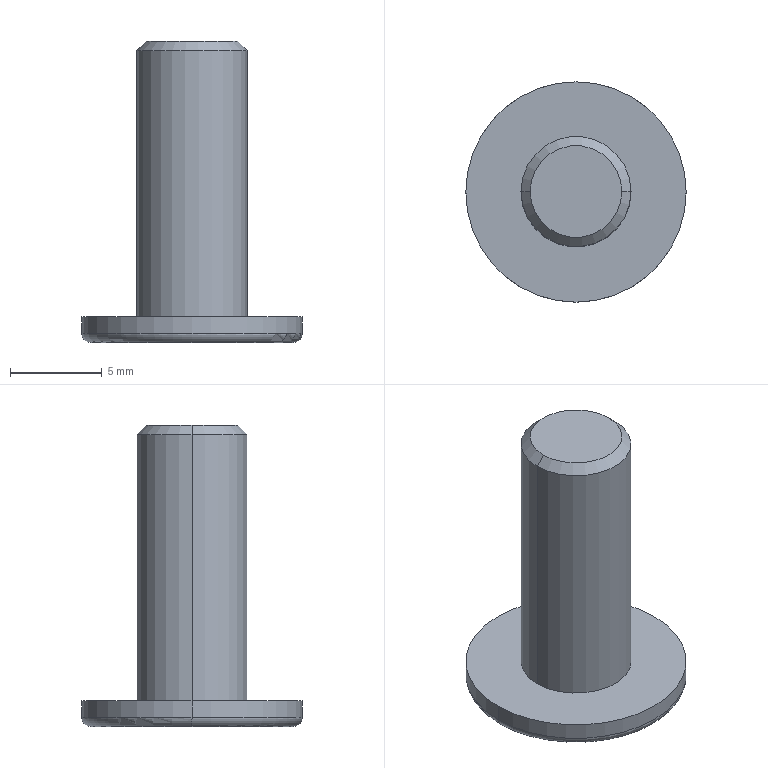Part | 1 solid | 18 faces | box 12 x 12 x 16.4 mm | volume 550.528 mm3 | plane 10 | cylinder 4 | cone 2 | torus 2 | commonest cylinder face diameters 6 x2 12 x2
STEP:
#1=CARTESIAN_POINT('',(2.5,0.,16.4));
#2=VERTEX_POINT('',#1);
#3=CARTESIAN_POINT('',(-2.5,0.,16.4));
#4=VERTEX_POINT('',#3);
#5=CARTESIAN_POINT('',(0.,0.,16.4));
#6=DIRECTION('',(0.,0.,1.));
#7=DIRECTION('',(1.,0.,0.));
#8=AXIS2_PLACEMENT_3D('',#5,#6,#7);
#9=CIRCLE('',#8,2.5);
#10=EDGE_CURVE('',#2,#4,#9,.T.);
#11=ORIENTED_EDGE('',*,*,#10,.F.);
#12=CARTESIAN_POINT('',(3.,0.,15.9));
#13=VERTEX_POINT('',#12);
#14=CARTESIAN_POINT('',(2.5,0.,16.4));
#15=DIRECTION('',(0.7071,0.,-0.7071));
#16=VECTOR('',#15,1000.);
#17=LINE('',#14,#16);
#18=EDGE_CURVE('',#2,#13,#17,.T.);
#19=ORIENTED_EDGE('',*,*,#18,.T.);
#20=CARTESIAN_POINT('',(-3.,0.,15.9));
#21=VERTEX_POINT('',#20);
#22=CARTESIAN_POINT('',(0.,0.,15.9));
#23=DIRECTION('',(0.,0.,-1.));
#24=DIRECTION('',(1.,0.,0.));
#25=AXIS2_PLACEMENT_3D('',#22,#23,#24);
#26=CIRCLE('',#25,3.);
#27=EDGE_CURVE('',#21,#13,#26,.T.);
#28=ORIENTED_EDGE('',*,*,#27,.F.);
#29=CARTESIAN_POINT('',(-2.5,0.,16.4));
#30=DIRECTION('',(-0.7071,0.,-0.7071));
#31=VECTOR('',#30,1000.);
#32=LINE('',#29,#31);
#33=EDGE_CURVE('',#4,#21,#32,.T.);
#34=ORIENTED_EDGE('',*,*,#33,.F.);
#35=EDGE_LOOP('',(#11,#19,#28,#34));
#36=FACE_OUTER_BOUND('',#35,.T.);
#37=CARTESIAN_POINT('',(0.,0.,16.4));
#38=DIRECTION('',(0.,0.,-1.));
#39=DIRECTION('',(-1.,0.,0.));
#40=AXIS2_PLACEMENT_3D('',#37,#38,#39);
#41=CONICAL_SURFACE('',#40,2.5,0.7854);
#42=ADVANCED_FACE('',(#36),#41,.T.);
#43=CARTESIAN_POINT('',(-5.5,0.,0.));
#44=VERTEX_POINT('',#43);
#45=CARTESIAN_POINT('',(5.5,0.,0.));
#46=VERTEX_POINT('',#45);
#47=CARTESIAN_POINT('',(0.,0.,0.));
#48=DIRECTION('',(0.,0.,-1.));
#49=DIRECTION('',(1.,0.,0.));
#50=AXIS2_PLACEMENT_3D('',#47,#48,#49);
#51=CIRCLE('',#50,5.5);
#52=EDGE_CURVE('',#44,#46,#51,.T.);
#53=ORIENTED_EDGE('',*,*,#52,.F.);
#54=CARTESIAN_POINT('',(-6.,0.,0.5));
#55=VERTEX_POINT('',#54);
#56=CARTESIAN_POINT('',(-5.5,0.,0.5));
#57=DIRECTION('',(0.,1.,0.));
#58=DIRECTION('',(-1.,0.,0.));
#59=AXIS2_PLACEMENT_3D('',#56,#57,#58);
#60=CIRCLE('',#59,0.5);
#61=EDGE_CURVE('',#44,#55,#60,.T.);
#62=ORIENTED_EDGE('',*,*,#61,.T.);
#63=CARTESIAN_POINT('',(6.,0.,0.5));
#64=VERTEX_POINT('',#63);
#65=CARTESIAN_POINT('',(0.,0.,0.5));
#66=DIRECTION('',(0.,0.,1.));
#67=DIRECTION('',(1.,0.,0.));
#68=AXIS2_PLACEMENT_3D('',#65,#66,#67);
#69=CIRCLE('',#68,6.);
#70=EDGE_CURVE('',#64,#55,#69,.T.);
#71=ORIENTED_EDGE('',*,*,#70,.F.);
#72=CARTESIAN_POINT('',(5.5,0.,0.5));
#73=DIRECTION('',(0.,-1.,0.));
#74=DIRECTION('',(0.,0.,-1.));
#75=AXIS2_PLACEMENT_3D('',#72,#73,#74);
#76=CIRCLE('',#75,0.5);
#77=EDGE_CURVE('',#46,#64,#76,.T.);
#78=ORIENTED_EDGE('',*,*,#77,.F.);
#79=EDGE_LOOP('',(#53,#62,#71,#78));
#80=FACE_OUTER_BOUND('',#79,.T.);
#81=CARTESIAN_POINT('',(0.,0.,0.5));
#82=DIRECTION('',(0.,0.,1.));
#83=DIRECTION('',(1.,0.,0.));
#84=AXIS2_PLACEMENT_3D('',#81,#82,#83);
#85=TOROIDAL_SURFACE('',#84,5.5,0.5);
#86=ADVANCED_FACE('',(#80),#85,.T.);
#87=ORIENTED_EDGE('',*,*,#27,.T.);
#88=CARTESIAN_POINT('',(3.,0.,1.4));
#89=VERTEX_POINT('',#88);
#90=CARTESIAN_POINT('',(3.,0.,16.4));
#91=DIRECTION('',(0.,0.,-1.));
#92=VECTOR('',#91,1000.);
#93=LINE('',#90,#92);
#94=EDGE_CURVE('',#13,#89,#93,.T.);
#95=ORIENTED_EDGE('',*,*,#94,.T.);
#96=CARTESIAN_POINT('',(-3.,0.,1.4));
#97=VERTEX_POINT('',#96);
#98=CARTESIAN_POINT('',(0.,0.,1.4));
#99=DIRECTION('',(0.,0.,1.));
#100=DIRECTION('',(1.,0.,0.));
#101=AXIS2_PLACEMENT_3D('',#98,#99,#100);
#102=CIRCLE('',#101,3.);
#103=EDGE_CURVE('',#89,#97,#102,.T.);
#104=ORIENTED_EDGE('',*,*,#103,.T.);
#105=CARTESIAN_POINT('',(-3.,0.,16.4));
#106=DIRECTION('',(0.,0.,-1.));
#107=VECTOR('',#106,1000.);
#108=LINE('',#105,#107);
#109=EDGE_CURVE('',#21,#97,#108,.T.);
#110=ORIENTED_EDGE('',*,*,#109,.F.);
#111=EDGE_LOOP('',(#87,#95,#104,#110));
#112=FACE_OUTER_BOUND('',#111,.T.);
#113=CARTESIAN_POINT('',(0.,0.,16.4));
#114=DIRECTION('',(0.,0.,-1.));
#115=DIRECTION('',(-1.,0.,0.));
#116=AXIS2_PLACEMENT_3D('',#113,#114,#115);
#117=CYLINDRICAL_SURFACE('',#116,3.);
#118=ADVANCED_FACE('',(#112),#117,.T.);
#119=CARTESIAN_POINT('',(6.,0.,1.4));
#120=VERTEX_POINT('',#119);
#121=CARTESIAN_POINT('',(-6.,0.,1.4));
#122=VERTEX_POINT('',#121);
#123=CARTESIAN_POINT('',(0.,0.,1.4));
#124=DIRECTION('',(0.,0.,1.));
#125=DIRECTION('',(1.,0.,0.));
#126=AXIS2_PLACEMENT_3D('',#123,#124,#125);
#127=CIRCLE('',#126,6.);
#128=EDGE_CURVE('',#120,#122,#127,.T.);
#129=ORIENTED_EDGE('',*,*,#128,.F.);
#130=CARTESIAN_POINT('',(6.,0.,1.4));
#131=DIRECTION('',(0.,0.,-1.));
#132=VECTOR('',#131,1000.);
#133=LINE('',#130,#132);
#134=EDGE_CURVE('',#120,#64,#133,.T.);
#135=ORIENTED_EDGE('',*,*,#134,.T.);
#136=ORIENTED_EDGE('',*,*,#70,.T.);
#137=CARTESIAN_POINT('',(-6.,0.,1.4));
#138=DIRECTION('',(0.,0.,-1.));
#139=VECTOR('',#138,1000.);
#140=LINE('',#137,#139);
#141=EDGE_CURVE('',#122,#55,#140,.T.);
#142=ORIENTED_EDGE('',*,*,#141,.F.);
#143=EDGE_LOOP('',(#129,#135,#136,#142));
#144=FACE_OUTER_BOUND('',#143,.T.);
#145=CARTESIAN_POINT('',(0.,0.,1.4));
#146=DIRECTION('',(0.,0.,-1.));
#147=DIRECTION('',(-1.,0.,0.));
#148=AXIS2_PLACEMENT_3D('',#145,#146,#147);
#149=CYLINDRICAL_SURFACE('',#148,6.);
#150=ADVANCED_FACE('',(#144),#149,.T.);
#151=ORIENTED_EDGE('',*,*,#134,.F.);
#152=CARTESIAN_POINT('',(0.,0.,1.4));
#153=DIRECTION('',(0.,0.,1.));
#154=DIRECTION('',(1.,0.,0.));
#155=AXIS2_PLACEMENT_3D('',#152,#153,#154);
#156=CIRCLE('',#155,6.);
#157=EDGE_CURVE('',#122,#120,#156,.T.);
#158=ORIENTED_EDGE('',*,*,#157,.F.);
#159=ORIENTED_EDGE('',*,*,#141,.T.);
#160=CARTESIAN_POINT('',(0.,0.,0.5));
#161=DIRECTION('',(0.,0.,1.));
#162=DIRECTION('',(1.,0.,0.));
#163=AXIS2_PLACEMENT_3D('',#160,#161,#162);
#164=CIRCLE('',#163,6.);
#165=EDGE_CURVE('',#55,#64,#164,.T.);
#166=ORIENTED_EDGE('',*,*,#165,.T.);
#167=EDGE_LOOP('',(#151,#158,#159,#166));
#168=FACE_OUTER_BOUND('',#167,.T.);
#169=CARTESIAN_POINT('',(0.,0.,1.4));
#170=DIRECTION('',(0.,0.,-1.));
#171=DIRECTION('',(-1.,0.,0.));
#172=AXIS2_PLACEMENT_3D('',#169,#170,#171);
#173=CYLINDRICAL_SURFACE('',#172,6.);
#174=ADVANCED_FACE('',(#168),#173,.T.);
#175=CARTESIAN_POINT('',(0.,0.,1.4));
#176=DIRECTION('',(0.,0.,1.));
#177=DIRECTION('',(1.,0.,0.));
#178=AXIS2_PLACEMENT_3D('',#175,#176,#177);
#179=CIRCLE('',#178,3.);
#180=EDGE_CURVE('',#97,#89,#179,.T.);
#181=ORIENTED_EDGE('',*,*,#180,.F.);
#182=ORIENTED_EDGE('',*,*,#103,.F.);
#183=EDGE_LOOP('',(#181,#182));
#184=FACE_BOUND('',#183,.T.);
#185=ORIENTED_EDGE('',*,*,#157,.T.);
#186=ORIENTED_EDGE('',*,*,#128,.T.);
#187=EDGE_LOOP('',(#185,#186));
#188=FACE_OUTER_BOUND('',#187,.T.);
#189=CARTESIAN_POINT('',(0.,0.,1.4));
#190=DIRECTION('',(0.,0.,1.));
#191=DIRECTION('',(1.,0.,0.));
#192=AXIS2_PLACEMENT_3D('',#189,#190,#191);
#193=PLANE('',#192);
#194=ADVANCED_FACE('',(#184,#188),#193,.T.);
#195=CARTESIAN_POINT('',(-0.7495,-2.184,0.));
#196=VERTEX_POINT('',#195);
#197=CARTESIAN_POINT('',(-2.267,-0.4431,0.));
#198=VERTEX_POINT('',#197);
#199=CARTESIAN_POINT('',(-0.7495,-2.184,0.));
#200=DIRECTION('',(-0.6569,0.754,0.));
#201=VECTOR('',#200,1000.);
#202=LINE('',#199,#201);
#203=EDGE_CURVE('',#196,#198,#202,.T.);
#204=ORIENTED_EDGE('',*,*,#203,.F.);
#205=CARTESIAN_POINT('',(1.517,-1.741,0.));
#206=VERTEX_POINT('',#205);
#207=CARTESIAN_POINT('',(1.517,-1.741,0.));
#208=DIRECTION('',(-0.9814,-0.1919,0.));
#209=VECTOR('',#208,1000.);
#210=LINE('',#207,#209);
#211=EDGE_CURVE('',#206,#196,#210,.T.);
#212=ORIENTED_EDGE('',*,*,#211,.F.);
#213=CARTESIAN_POINT('',(2.267,0.4431,0.));
#214=VERTEX_POINT('',#213);
#215=CARTESIAN_POINT('',(2.267,0.4431,0.));
#216=DIRECTION('',(-0.3246,-0.9459,0.));
#217=VECTOR('',#216,1000.);
#218=LINE('',#215,#217);
#219=EDGE_CURVE('',#214,#206,#218,.T.);
#220=ORIENTED_EDGE('',*,*,#219,.F.);
#221=CARTESIAN_POINT('',(0.7495,2.184,0.));
#222=VERTEX_POINT('',#221);
#223=CARTESIAN_POINT('',(0.7495,2.184,0.));
#224=DIRECTION('',(0.6569,-0.754,0.));
#225=VECTOR('',#224,1000.);
#226=LINE('',#223,#225);
#227=EDGE_CURVE('',#222,#214,#226,.T.);
#228=ORIENTED_EDGE('',*,*,#227,.F.);
#229=CARTESIAN_POINT('',(-1.517,1.741,0.));
#230=VERTEX_POINT('',#229);
#231=CARTESIAN_POINT('',(-1.517,1.741,0.));
#232=DIRECTION('',(0.9814,0.1919,0.));
#233=VECTOR('',#232,1000.);
#234=LINE('',#231,#233);
#235=EDGE_CURVE('',#230,#222,#234,.T.);
#236=ORIENTED_EDGE('',*,*,#235,.F.);
#237=CARTESIAN_POINT('',(-2.267,-0.4431,0.));
#238=DIRECTION('',(0.3246,0.9459,0.));
#239=VECTOR('',#238,1000.);
#240=LINE('',#237,#239);
#241=EDGE_CURVE('',#198,#230,#240,.T.);
#242=ORIENTED_EDGE('',*,*,#241,.F.);
#243=EDGE_LOOP('',(#204,#212,#220,#228,#236,#242));
#244=FACE_BOUND('',#243,.T.);
#245=CARTESIAN_POINT('',(0.,0.,0.));
#246=DIRECTION('',(0.,0.,-1.));
#247=DIRECTION('',(1.,0.,0.));
#248=AXIS2_PLACEMENT_3D('',#245,#246,#247);
#249=CIRCLE('',#248,5.5);
#250=EDGE_CURVE('',#46,#44,#249,.T.);
#251=ORIENTED_EDGE('',*,*,#250,.T.);
#252=ORIENTED_EDGE('',*,*,#52,.T.);
#253=EDGE_LOOP('',(#251,#252));
#254=FACE_OUTER_BOUND('',#253,.T.);
#255=CARTESIAN_POINT('',(0.,0.,0.));
#256=DIRECTION('',(0.,0.,1.));
#257=DIRECTION('',(1.,0.,0.));
#258=AXIS2_PLACEMENT_3D('',#255,#256,#257);
#259=PLANE('',#258);
#260=ADVANCED_FACE('',(#244,#254),#259,.F.);
#261=ORIENTED_EDGE('',*,*,#94,.F.);
#262=CARTESIAN_POINT('',(0.,0.,15.9));
#263=DIRECTION('',(0.,0.,-1.));
#264=DIRECTION('',(1.,0.,0.));
#265=AXIS2_PLACEMENT_3D('',#262,#263,#264);
#266=CIRCLE('',#265,3.);
#267=EDGE_CURVE('',#13,#21,#266,.T.);
#268=ORIENTED_EDGE('',*,*,#267,.T.);
#269=ORIENTED_EDGE('',*,*,#109,.T.);
#270=ORIENTED_EDGE('',*,*,#180,.T.);
#271=EDGE_LOOP('',(#261,#268,#269,#270));
#272=FACE_OUTER_BOUND('',#271,.T.);
#273=CARTESIAN_POINT('',(0.,0.,16.4));
#274=DIRECTION('',(0.,0.,-1.));
#275=DIRECTION('',(-1.,0.,0.));
#276=AXIS2_PLACEMENT_3D('',#273,#274,#275);
#277=CYLINDRICAL_SURFACE('',#276,3.);
#278=ADVANCED_FACE('',(#272),#277,.T.);
#279=CARTESIAN_POINT('',(0.,0.,16.4));
#280=DIRECTION('',(0.,0.,1.));
#281=DIRECTION('',(1.,0.,0.));
#282=AXIS2_PLACEMENT_3D('',#279,#280,#281);
#283=CIRCLE('',#282,2.5);
#284=EDGE_CURVE('',#4,#2,#283,.T.);
#285=ORIENTED_EDGE('',*,*,#284,.T.);
#286=ORIENTED_EDGE('',*,*,#10,.T.);
#287=EDGE_LOOP('',(#285,#286));
#288=FACE_OUTER_BOUND('',#287,.T.);
#289=CARTESIAN_POINT('',(0.,0.,16.4));
#290=DIRECTION('',(0.,0.,1.));
#291=DIRECTION('',(1.,0.,0.));
#292=AXIS2_PLACEMENT_3D('',#289,#290,#291);
#293=PLANE('',#292);
#294=ADVANCED_FACE('',(#288),#293,.T.);
#295=ORIENTED_EDGE('',*,*,#61,.F.);
#296=ORIENTED_EDGE('',*,*,#250,.F.);
#297=ORIENTED_EDGE('',*,*,#77,.T.);
#298=ORIENTED_EDGE('',*,*,#165,.F.);
#299=EDGE_LOOP('',(#295,#296,#297,#298));
#300=FACE_OUTER_BOUND('',#299,.T.);
#301=CARTESIAN_POINT('',(0.,0.,0.5));
#302=DIRECTION('',(0.,0.,1.));
#303=DIRECTION('',(1.,0.,0.));
#304=AXIS2_PLACEMENT_3D('',#301,#302,#303);
#305=TOROIDAL_SURFACE('',#304,5.5,0.5);
#306=ADVANCED_FACE('',(#300),#305,.T.);
#307=ORIENTED_EDGE('',*,*,#211,.T.);
#308=CARTESIAN_POINT('',(-0.7495,-2.184,2.));
#309=VERTEX_POINT('',#308);
#310=CARTESIAN_POINT('',(-0.7495,-2.184,2.));
#311=DIRECTION('',(0.,0.,-1.));
#312=VECTOR('',#311,1000.);
#313=LINE('',#310,#312);
#314=EDGE_CURVE('',#309,#196,#313,.T.);
#315=ORIENTED_EDGE('',*,*,#314,.F.);
#316=CARTESIAN_POINT('',(1.517,-1.741,2.));
#317=VERTEX_POINT('',#316);
#318=CARTESIAN_POINT('',(1.517,-1.741,2.));
#319=DIRECTION('',(-0.9814,-0.1919,0.));
#320=VECTOR('',#319,1000.);
#321=LINE('',#318,#320);
#322=EDGE_CURVE('',#317,#309,#321,.T.);
#323=ORIENTED_EDGE('',*,*,#322,.F.);
#324=CARTESIAN_POINT('',(1.517,-1.741,2.));
#325=DIRECTION('',(0.,0.,-1.));
#326=VECTOR('',#325,1000.);
#327=LINE('',#324,#326);
#328=EDGE_CURVE('',#317,#206,#327,.T.);
#329=ORIENTED_EDGE('',*,*,#328,.T.);
#330=EDGE_LOOP('',(#307,#315,#323,#329));
#331=FACE_OUTER_BOUND('',#330,.T.);
#332=CARTESIAN_POINT('',(1.517,-1.741,2.));
#333=DIRECTION('',(0.1919,-0.9814,0.));
#334=DIRECTION('',(0.9814,0.1919,0.));
#335=AXIS2_PLACEMENT_3D('',#332,#333,#334);
#336=PLANE('',#335);
#337=ADVANCED_FACE('',(#331),#336,.F.);
#338=ORIENTED_EDGE('',*,*,#219,.T.);
#339=ORIENTED_EDGE('',*,*,#328,.F.);
#340=CARTESIAN_POINT('',(2.267,0.4431,2.));
#341=VERTEX_POINT('',#340);
#342=CARTESIAN_POINT('',(2.267,0.4431,2.));
#343=DIRECTION('',(-0.3246,-0.9459,0.));
#344=VECTOR('',#343,1000.);
#345=LINE('',#342,#344);
#346=EDGE_CURVE('',#341,#317,#345,.T.);
#347=ORIENTED_EDGE('',*,*,#346,.F.);
#348=CARTESIAN_POINT('',(2.267,0.4431,2.));
#349=DIRECTION('',(0.,0.,-1.));
#350=VECTOR('',#349,1000.);
#351=LINE('',#348,#350);
#352=EDGE_CURVE('',#341,#214,#351,.T.);
#353=ORIENTED_EDGE('',*,*,#352,.T.);
#354=EDGE_LOOP('',(#338,#339,#347,#353));
#355=FACE_OUTER_BOUND('',#354,.T.);
#356=CARTESIAN_POINT('',(2.267,0.4431,2.));
#357=DIRECTION('',(0.9459,-0.3246,0.));
#358=DIRECTION('',(0.3246,0.9459,0.));
#359=AXIS2_PLACEMENT_3D('',#356,#357,#358);
#360=PLANE('',#359);
#361=ADVANCED_FACE('',(#355),#360,.F.);
#362=ORIENTED_EDGE('',*,*,#227,.T.);
#363=ORIENTED_EDGE('',*,*,#352,.F.);
#364=CARTESIAN_POINT('',(0.7495,2.184,2.));
#365=VERTEX_POINT('',#364);
#366=CARTESIAN_POINT('',(0.7495,2.184,2.));
#367=DIRECTION('',(0.6569,-0.754,0.));
#368=VECTOR('',#367,1000.);
#369=LINE('',#366,#368);
#370=EDGE_CURVE('',#365,#341,#369,.T.);
#371=ORIENTED_EDGE('',*,*,#370,.F.);
#372=CARTESIAN_POINT('',(0.7495,2.184,2.));
#373=DIRECTION('',(0.,0.,-1.));
#374=VECTOR('',#373,1000.);
#375=LINE('',#372,#374);
#376=EDGE_CURVE('',#365,#222,#375,.T.);
#377=ORIENTED_EDGE('',*,*,#376,.T.);
#378=EDGE_LOOP('',(#362,#363,#371,#377));
#379=FACE_OUTER_BOUND('',#378,.T.);
#380=CARTESIAN_POINT('',(0.7495,2.184,2.));
#381=DIRECTION('',(0.754,0.6569,0.));
#382=DIRECTION('',(-0.6569,0.754,0.));
#383=AXIS2_PLACEMENT_3D('',#380,#381,#382);
#384=PLANE('',#383);
#385=ADVANCED_FACE('',(#379),#384,.F.);
#386=ORIENTED_EDGE('',*,*,#235,.T.);
#387=ORIENTED_EDGE('',*,*,#376,.F.);
#388=CARTESIAN_POINT('',(-1.517,1.741,2.));
#389=VERTEX_POINT('',#388);
#390=CARTESIAN_POINT('',(-1.517,1.741,2.));
#391=DIRECTION('',(0.9814,0.1919,0.));
#392=VECTOR('',#391,1000.);
#393=LINE('',#390,#392);
#394=EDGE_CURVE('',#389,#365,#393,.T.);
#395=ORIENTED_EDGE('',*,*,#394,.F.);
#396=CARTESIAN_POINT('',(-1.517,1.741,2.));
#397=DIRECTION('',(0.,0.,-1.));
#398=VECTOR('',#397,1000.);
#399=LINE('',#396,#398);
#400=EDGE_CURVE('',#389,#230,#399,.T.);
#401=ORIENTED_EDGE('',*,*,#400,.T.);
#402=EDGE_LOOP('',(#386,#387,#395,#401));
#403=FACE_OUTER_BOUND('',#402,.T.);
#404=CARTESIAN_POINT('',(-1.517,1.741,2.));
#405=DIRECTION('',(-0.1919,0.9814,0.));
#406=DIRECTION('',(-0.9814,-0.1919,0.));
#407=AXIS2_PLACEMENT_3D('',#404,#405,#406);
#408=PLANE('',#407);
#409=ADVANCED_FACE('',(#403),#408,.F.);
#410=ORIENTED_EDGE('',*,*,#241,.T.);
#411=ORIENTED_EDGE('',*,*,#400,.F.);
#412=CARTESIAN_POINT('',(-2.267,-0.4431,2.));
#413=VERTEX_POINT('',#412);
#414=CARTESIAN_POINT('',(-2.267,-0.4431,2.));
#415=DIRECTION('',(0.3246,0.9459,0.));
#416=VECTOR('',#415,1000.);
#417=LINE('',#414,#416);
#418=EDGE_CURVE('',#413,#389,#417,.T.);
#419=ORIENTED_EDGE('',*,*,#418,.F.);
#420=CARTESIAN_POINT('',(-2.267,-0.4431,2.));
#421=DIRECTION('',(0.,0.,-1.));
#422=VECTOR('',#421,1000.);
#423=LINE('',#420,#422);
#424=EDGE_CURVE('',#413,#198,#423,.T.);
#425=ORIENTED_EDGE('',*,*,#424,.T.);
#426=EDGE_LOOP('',(#410,#411,#419,#425));
#427=FACE_OUTER_BOUND('',#426,.T.);
#428=CARTESIAN_POINT('',(-2.267,-0.4431,2.));
#429=DIRECTION('',(-0.9459,0.3246,0.));
#430=DIRECTION('',(-0.3246,-0.9459,0.));
#431=AXIS2_PLACEMENT_3D('',#428,#429,#430);
#432=PLANE('',#431);
#433=ADVANCED_FACE('',(#427),#432,.F.);
#434=ORIENTED_EDGE('',*,*,#203,.T.);
#435=ORIENTED_EDGE('',*,*,#424,.F.);
#436=CARTESIAN_POINT('',(-0.7495,-2.184,2.));
#437=DIRECTION('',(-0.6569,0.754,0.));
#438=VECTOR('',#437,1000.);
#439=LINE('',#436,#438);
#440=EDGE_CURVE('',#309,#413,#439,.T.);
#441=ORIENTED_EDGE('',*,*,#440,.F.);
#442=ORIENTED_EDGE('',*,*,#314,.T.);
#443=EDGE_LOOP('',(#434,#435,#441,#442));
#444=FACE_OUTER_BOUND('',#443,.T.);
#445=CARTESIAN_POINT('',(-0.7495,-2.184,2.));
#446=DIRECTION('',(-0.754,-0.6569,0.));
#447=DIRECTION('',(0.6569,-0.754,0.));
#448=AXIS2_PLACEMENT_3D('',#445,#446,#447);
#449=PLANE('',#448);
#450=ADVANCED_FACE('',(#444),#449,.F.);
#451=ORIENTED_EDGE('',*,*,#322,.T.);
#452=ORIENTED_EDGE('',*,*,#440,.T.);
#453=ORIENTED_EDGE('',*,*,#418,.T.);
#454=ORIENTED_EDGE('',*,*,#394,.T.);
#455=ORIENTED_EDGE('',*,*,#370,.T.);
#456=ORIENTED_EDGE('',*,*,#346,.T.);
#457=EDGE_LOOP('',(#451,#452,#453,#454,#455,#456));
#458=FACE_OUTER_BOUND('',#457,.T.);
#459=CARTESIAN_POINT('',(0.,0.,2.));
#460=DIRECTION('',(0.,0.,-1.));
#461=DIRECTION('',(-1.,0.,0.));
#462=AXIS2_PLACEMENT_3D('',#459,#460,#461);
#463=PLANE('',#462);
#464=ADVANCED_FACE('',(#458),#463,.T.);
#465=ORIENTED_EDGE('',*,*,#18,.F.);
#466=ORIENTED_EDGE('',*,*,#284,.F.);
#467=ORIENTED_EDGE('',*,*,#33,.T.);
#468=ORIENTED_EDGE('',*,*,#267,.F.);
#469=EDGE_LOOP('',(#465,#466,#467,#468));
#470=FACE_OUTER_BOUND('',#469,.T.);
#471=CARTESIAN_POINT('',(0.,0.,16.4));
#472=DIRECTION('',(0.,0.,-1.));
#473=DIRECTION('',(-1.,0.,0.));
#474=AXIS2_PLACEMENT_3D('',#471,#472,#473);
#475=CONICAL_SURFACE('',#474,2.5,0.7854);
#476=ADVANCED_FACE('',(#470),#475,.T.);
#477=CLOSED_SHELL('',(#42,#86,#118,#150,#174,#194,#260,#278,#294,#306,#337,#361,#385,#409,#433,#450,#464,#476));
#478=MANIFOLD_SOLID_BREP('',#477);
#479=CARTESIAN_POINT('',(0.,0.,0.));
#480=DIRECTION('',(0.,0.,1.));
#481=DIRECTION('',(1.,0.,0.));
#482=AXIS2_PLACEMENT_3D('',#479,#480,#481);
#483=(LENGTH_UNIT()NAMED_UNIT(*)SI_UNIT(.MILLI.,.METRE.));
#484=UNCERTAINTY_MEASURE_WITH_UNIT(LENGTH_MEASURE(0.00001),#483,'','');
#485=(NAMED_UNIT(*)PLANE_ANGLE_UNIT()SI_UNIT($,.RADIAN.));
#486=(NAMED_UNIT(*)SI_UNIT($,.STERADIAN.)SOLID_ANGLE_UNIT());
#487=(GEOMETRIC_REPRESENTATION_CONTEXT(3)GLOBAL_UNCERTAINTY_ASSIGNED_CONTEXT((#484))GLOBAL_UNIT_ASSIGNED_CONTEXT((#483,#485,#486))REPRESENTATION_CONTEXT('',''));
#488=ADVANCED_BREP_SHAPE_REPRESENTATION('',(#478,#482),#487);